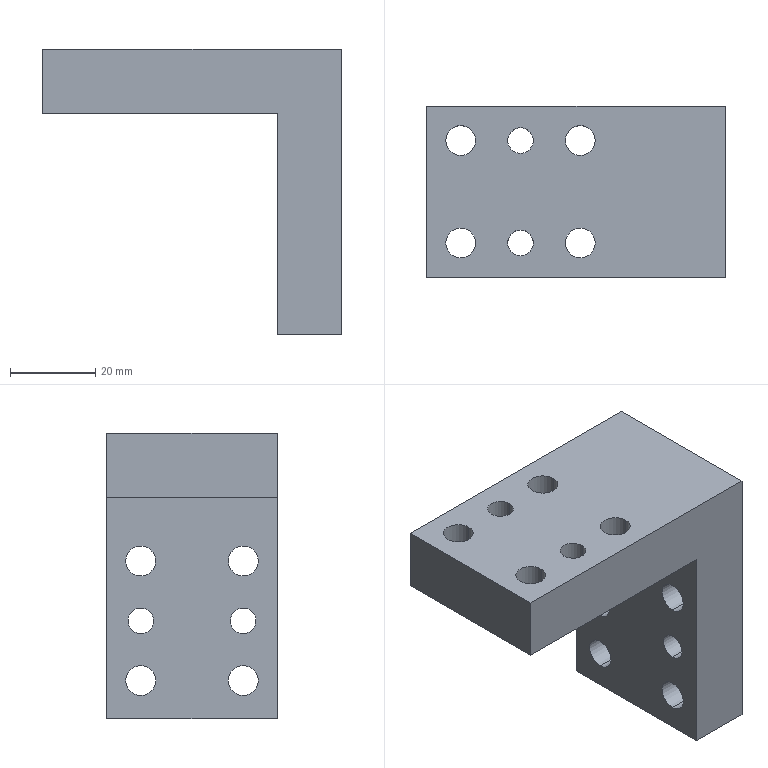Part | STEP file | Positioning_id1522_x_t | 1 solid | 32 faces | box 70 x 40 x 67 mm | volume 66885 mm3 | cylinder 24 | plane 8 | commonest cylinder face diameters 7 x16 6 x8